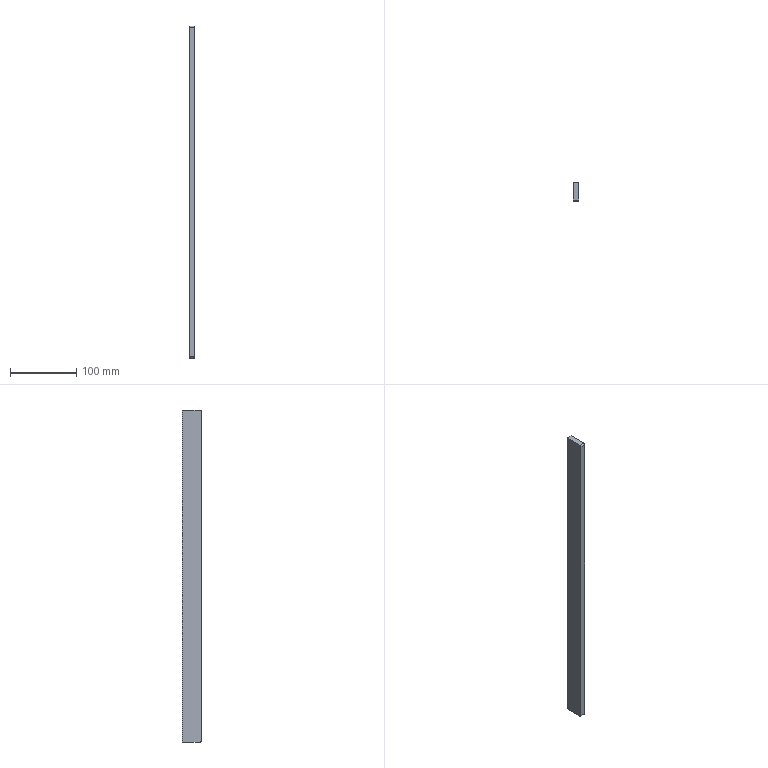Part | SolidWorks | features BaseBody 1 | 1 solid | 20 faces | box 8 x 29 x 500 mm | volume 115683 mm3 | cylinder 8 | cone 6 | plane 6 | commonest cylinder face diameters 3.3 x6 4 x2
STEP:
#1=CARTESIAN_POINT('',(-38.606,219.931,3066.293));
#2=VERTEX_POINT('',#1);
#3=CARTESIAN_POINT('',(-35.306,219.931,3066.293));
#4=VERTEX_POINT('',#3);
#5=CARTESIAN_POINT('',(-36.956,219.931,3066.293));
#6=DIRECTION('',(0.,1.,0.));
#7=DIRECTION('',(1.,0.,0.));
#8=AXIS2_PLACEMENT_3D('',#5,#6,#7);
#9=CIRCLE('',#8,1.65);
#10=EDGE_CURVE('',#2,#4,#9,.T.);
#11=ORIENTED_EDGE('',*,*,#10,.F.);
#12=CARTESIAN_POINT('',(-38.606,231.431,3066.293));
#13=VERTEX_POINT('',#12);
#14=CARTESIAN_POINT('',(-38.606,231.431,3066.293));
#15=DIRECTION('',(0.,1.,0.));
#16=VECTOR('',#15,1000.);
#17=LINE('',#14,#16);
#18=EDGE_CURVE('',#2,#13,#17,.T.);
#19=ORIENTED_EDGE('',*,*,#18,.T.);
#20=CARTESIAN_POINT('',(-35.306,231.431,3066.293));
#21=VERTEX_POINT('',#20);
#22=CARTESIAN_POINT('',(-36.956,231.431,3066.293));
#23=DIRECTION('',(0.,1.,0.));
#24=DIRECTION('',(1.,0.,0.));
#25=AXIS2_PLACEMENT_3D('',#22,#23,#24);
#26=CIRCLE('',#25,1.65);
#27=EDGE_CURVE('',#13,#21,#26,.T.);
#28=ORIENTED_EDGE('',*,*,#27,.T.);
#29=CARTESIAN_POINT('',(-35.306,231.431,3066.293));
#30=DIRECTION('',(0.,1.,0.));
#31=VECTOR('',#30,1000.);
#32=LINE('',#29,#31);
#33=EDGE_CURVE('',#4,#21,#32,.T.);
#34=ORIENTED_EDGE('',*,*,#33,.F.);
#35=EDGE_LOOP('',(#11,#19,#28,#34));
#36=FACE_OUTER_BOUND('',#35,.T.);
#37=CARTESIAN_POINT('',(-36.956,231.431,3066.293));
#38=DIRECTION('',(0.,1.,0.));
#39=DIRECTION('',(1.,0.,0.));
#40=AXIS2_PLACEMENT_3D('',#37,#38,#39);
#41=CYLINDRICAL_SURFACE('',#40,1.65);
#42=ADVANCED_FACE('',(#36),#41,.F.);
#43=CARTESIAN_POINT('',(-36.956,218.94,3066.293));
#44=VERTEX_POINT('',#43);
#45=CARTESIAN_POINT('',(-35.306,219.931,3066.293));
#46=DIRECTION('',(0.8572,0.515,0.));
#47=VECTOR('',#46,1000.);
#48=LINE('',#45,#47);
#49=EDGE_CURVE('',#44,#4,#48,.T.);
#50=ORIENTED_EDGE('',*,*,#49,.F.);
#51=CARTESIAN_POINT('',(-38.606,219.931,3066.293));
#52=DIRECTION('',(-0.8572,0.515,0.));
#53=VECTOR('',#52,1000.);
#54=LINE('',#51,#53);
#55=EDGE_CURVE('',#44,#2,#54,.T.);
#56=ORIENTED_EDGE('',*,*,#55,.T.);
#57=ORIENTED_EDGE('',*,*,#10,.T.);
#58=EDGE_LOOP('',(#50,#56,#57));
#59=FACE_OUTER_BOUND('',#58,.T.);
#60=CARTESIAN_POINT('',(-36.956,219.931,3066.293));
#61=DIRECTION('',(0.,1.,0.));
#62=DIRECTION('',(1.,0.,0.));
#63=AXIS2_PLACEMENT_3D('',#60,#61,#62);
#64=CONICAL_SURFACE('',#63,1.65,1.03);
#65=ADVANCED_FACE('',(#59),#64,.F.);
#66=CARTESIAN_POINT('',(-38.606,219.931,2596.293));
#67=VERTEX_POINT('',#66);
#68=CARTESIAN_POINT('',(-35.306,219.931,2596.293));
#69=VERTEX_POINT('',#68);
#70=CARTESIAN_POINT('',(-36.956,219.931,2596.293));
#71=DIRECTION('',(0.,1.,0.));
#72=DIRECTION('',(1.,0.,0.));
#73=AXIS2_PLACEMENT_3D('',#70,#71,#72);
#74=CIRCLE('',#73,1.65);
#75=EDGE_CURVE('',#67,#69,#74,.T.);
#76=ORIENTED_EDGE('',*,*,#75,.F.);
#77=CARTESIAN_POINT('',(-38.606,231.431,2596.293));
#78=VERTEX_POINT('',#77);
#79=CARTESIAN_POINT('',(-38.606,231.431,2596.293));
#80=DIRECTION('',(0.,1.,0.));
#81=VECTOR('',#80,1000.);
#82=LINE('',#79,#81);
#83=EDGE_CURVE('',#67,#78,#82,.T.);
#84=ORIENTED_EDGE('',*,*,#83,.T.);
#85=CARTESIAN_POINT('',(-35.306,231.431,2596.293));
#86=VERTEX_POINT('',#85);
#87=CARTESIAN_POINT('',(-36.956,231.431,2596.293));
#88=DIRECTION('',(0.,1.,0.));
#89=DIRECTION('',(1.,0.,0.));
#90=AXIS2_PLACEMENT_3D('',#87,#88,#89);
#91=CIRCLE('',#90,1.65);
#92=EDGE_CURVE('',#78,#86,#91,.T.);
#93=ORIENTED_EDGE('',*,*,#92,.T.);
#94=CARTESIAN_POINT('',(-35.306,231.431,2596.293));
#95=DIRECTION('',(0.,1.,0.));
#96=VECTOR('',#95,1000.);
#97=LINE('',#94,#96);
#98=EDGE_CURVE('',#69,#86,#97,.T.);
#99=ORIENTED_EDGE('',*,*,#98,.F.);
#100=EDGE_LOOP('',(#76,#84,#93,#99));
#101=FACE_OUTER_BOUND('',#100,.T.);
#102=CARTESIAN_POINT('',(-36.956,231.431,2596.293));
#103=DIRECTION('',(0.,1.,0.));
#104=DIRECTION('',(1.,0.,0.));
#105=AXIS2_PLACEMENT_3D('',#102,#103,#104);
#106=CYLINDRICAL_SURFACE('',#105,1.65);
#107=ADVANCED_FACE('',(#101),#106,.F.);
#108=CARTESIAN_POINT('',(-36.956,218.94,2596.293));
#109=VERTEX_POINT('',#108);
#110=CARTESIAN_POINT('',(-35.306,219.931,2596.293));
#111=DIRECTION('',(0.8572,0.515,0.));
#112=VECTOR('',#111,1000.);
#113=LINE('',#110,#112);
#114=EDGE_CURVE('',#109,#69,#113,.T.);
#115=ORIENTED_EDGE('',*,*,#114,.F.);
#116=CARTESIAN_POINT('',(-38.606,219.931,2596.293));
#117=DIRECTION('',(-0.8572,0.515,0.));
#118=VECTOR('',#117,1000.);
#119=LINE('',#116,#118);
#120=EDGE_CURVE('',#109,#67,#119,.T.);
#121=ORIENTED_EDGE('',*,*,#120,.T.);
#122=ORIENTED_EDGE('',*,*,#75,.T.);
#123=EDGE_LOOP('',(#115,#121,#122));
#124=FACE_OUTER_BOUND('',#123,.T.);
#125=CARTESIAN_POINT('',(-36.956,219.931,2596.293));
#126=DIRECTION('',(0.,1.,0.));
#127=DIRECTION('',(1.,0.,0.));
#128=AXIS2_PLACEMENT_3D('',#125,#126,#127);
#129=CONICAL_SURFACE('',#128,1.65,1.03);
#130=ADVANCED_FACE('',(#124),#129,.F.);
#131=CARTESIAN_POINT('',(-38.606,219.931,2888.793));
#132=VERTEX_POINT('',#131);
#133=CARTESIAN_POINT('',(-35.306,219.931,2888.793));
#134=VERTEX_POINT('',#133);
#135=CARTESIAN_POINT('',(-36.956,219.931,2888.793));
#136=DIRECTION('',(0.,1.,0.));
#137=DIRECTION('',(1.,0.,0.));
#138=AXIS2_PLACEMENT_3D('',#135,#136,#137);
#139=CIRCLE('',#138,1.65);
#140=EDGE_CURVE('',#132,#134,#139,.T.);
#141=ORIENTED_EDGE('',*,*,#140,.F.);
#142=CARTESIAN_POINT('',(-38.606,231.431,2888.793));
#143=VERTEX_POINT('',#142);
#144=CARTESIAN_POINT('',(-38.606,231.431,2888.793));
#145=DIRECTION('',(0.,1.,0.));
#146=VECTOR('',#145,1000.);
#147=LINE('',#144,#146);
#148=EDGE_CURVE('',#132,#143,#147,.T.);
#149=ORIENTED_EDGE('',*,*,#148,.T.);
#150=CARTESIAN_POINT('',(-35.306,231.431,2888.793));
#151=VERTEX_POINT('',#150);
#152=CARTESIAN_POINT('',(-36.956,231.431,2888.793));
#153=DIRECTION('',(0.,1.,0.));
#154=DIRECTION('',(1.,0.,0.));
#155=AXIS2_PLACEMENT_3D('',#152,#153,#154);
#156=CIRCLE('',#155,1.65);
#157=EDGE_CURVE('',#143,#151,#156,.T.);
#158=ORIENTED_EDGE('',*,*,#157,.T.);
#159=CARTESIAN_POINT('',(-35.306,231.431,2888.793));
#160=DIRECTION('',(0.,1.,0.));
#161=VECTOR('',#160,1000.);
#162=LINE('',#159,#161);
#163=EDGE_CURVE('',#134,#151,#162,.T.);
#164=ORIENTED_EDGE('',*,*,#163,.F.);
#165=EDGE_LOOP('',(#141,#149,#158,#164));
#166=FACE_OUTER_BOUND('',#165,.T.);
#167=CARTESIAN_POINT('',(-36.956,231.431,2888.793));
#168=DIRECTION('',(0.,1.,0.));
#169=DIRECTION('',(1.,0.,0.));
#170=AXIS2_PLACEMENT_3D('',#167,#168,#169);
#171=CYLINDRICAL_SURFACE('',#170,1.65);
#172=ADVANCED_FACE('',(#166),#171,.F.);
#173=CARTESIAN_POINT('',(-36.956,218.94,2888.793));
#174=VERTEX_POINT('',#173);
#175=CARTESIAN_POINT('',(-35.306,219.931,2888.793));
#176=DIRECTION('',(0.8572,0.515,0.));
#177=VECTOR('',#176,1000.);
#178=LINE('',#175,#177);
#179=EDGE_CURVE('',#174,#134,#178,.T.);
#180=ORIENTED_EDGE('',*,*,#179,.F.);
#181=CARTESIAN_POINT('',(-38.606,219.931,2888.793));
#182=DIRECTION('',(-0.8572,0.515,0.));
#183=VECTOR('',#182,1000.);
#184=LINE('',#181,#183);
#185=EDGE_CURVE('',#174,#132,#184,.T.);
#186=ORIENTED_EDGE('',*,*,#185,.T.);
#187=ORIENTED_EDGE('',*,*,#140,.T.);
#188=EDGE_LOOP('',(#180,#186,#187));
#189=FACE_OUTER_BOUND('',#188,.T.);
#190=CARTESIAN_POINT('',(-36.956,219.931,2888.793));
#191=DIRECTION('',(0.,1.,0.));
#192=DIRECTION('',(1.,0.,0.));
#193=AXIS2_PLACEMENT_3D('',#190,#191,#192);
#194=CONICAL_SURFACE('',#193,1.65,1.03);
#195=ADVANCED_FACE('',(#189),#194,.F.);
#196=CARTESIAN_POINT('',(-32.956,204.431,2581.293));
#197=VERTEX_POINT('',#196);
#198=CARTESIAN_POINT('',(-32.956,231.431,2581.293));
#199=VERTEX_POINT('',#198);
#200=CARTESIAN_POINT('',(-32.956,231.431,2581.293));
#201=DIRECTION('',(0.,1.,0.));
#202=VECTOR('',#201,1000.);
#203=LINE('',#200,#202);
#204=EDGE_CURVE('',#197,#199,#203,.T.);
#205=ORIENTED_EDGE('',*,*,#204,.F.);
#206=CARTESIAN_POINT('',(-40.956,204.431,2581.293));
#207=VERTEX_POINT('',#206);
#208=CARTESIAN_POINT('',(-32.956,204.431,2581.293));
#209=DIRECTION('',(-1.,0.,0.));
#210=VECTOR('',#209,1000.);
#211=LINE('',#208,#210);
#212=EDGE_CURVE('',#197,#207,#211,.T.);
#213=ORIENTED_EDGE('',*,*,#212,.T.);
#214=CARTESIAN_POINT('',(-40.956,231.431,2581.293));
#215=VERTEX_POINT('',#214);
#216=CARTESIAN_POINT('',(-40.956,231.431,2581.293));
#217=DIRECTION('',(0.,1.,0.));
#218=VECTOR('',#217,1000.);
#219=LINE('',#216,#218);
#220=EDGE_CURVE('',#207,#215,#219,.T.);
#221=ORIENTED_EDGE('',*,*,#220,.T.);
#222=CARTESIAN_POINT('',(-32.956,231.431,2581.293));
#223=DIRECTION('',(-1.,0.,0.));
#224=VECTOR('',#223,1000.);
#225=LINE('',#222,#224);
#226=EDGE_CURVE('',#199,#215,#225,.T.);
#227=ORIENTED_EDGE('',*,*,#226,.F.);
#228=EDGE_LOOP('',(#205,#213,#221,#227));
#229=FACE_OUTER_BOUND('',#228,.T.);
#230=CARTESIAN_POINT('',(-32.956,231.431,2581.293));
#231=DIRECTION('',(0.,0.,1.));
#232=DIRECTION('',(1.,0.,0.));
#233=AXIS2_PLACEMENT_3D('',#230,#231,#232);
#234=PLANE('',#233);
#235=ADVANCED_FACE('',(#229),#234,.F.);
#236=CARTESIAN_POINT('',(-40.956,231.431,3081.293));
#237=VERTEX_POINT('',#236);
#238=CARTESIAN_POINT('',(-40.956,231.431,3081.293));
#239=DIRECTION('',(0.,0.,1.));
#240=VECTOR('',#239,1000.);
#241=LINE('',#238,#240);
#242=EDGE_CURVE('',#215,#237,#241,.T.);
#243=ORIENTED_EDGE('',*,*,#242,.T.);
#244=CARTESIAN_POINT('',(-32.956,231.431,3081.293));
#245=VERTEX_POINT('',#244);
#246=CARTESIAN_POINT('',(-32.956,231.431,3081.293));
#247=DIRECTION('',(-1.,0.,0.));
#248=VECTOR('',#247,1000.);
#249=LINE('',#246,#248);
#250=EDGE_CURVE('',#245,#237,#249,.T.);
#251=ORIENTED_EDGE('',*,*,#250,.F.);
#252=CARTESIAN_POINT('',(-32.956,231.431,3081.293));
#253=DIRECTION('',(0.,0.,1.));
#254=VECTOR('',#253,1000.);
#255=LINE('',#252,#254);
#256=EDGE_CURVE('',#199,#245,#255,.T.);
#257=ORIENTED_EDGE('',*,*,#256,.F.);
#258=ORIENTED_EDGE('',*,*,#226,.T.);
#259=EDGE_LOOP('',(#243,#251,#257,#258));
#260=FACE_OUTER_BOUND('',#259,.T.);
#261=CARTESIAN_POINT('',(-36.956,231.431,3066.293));
#262=DIRECTION('',(0.,1.,0.));
#263=DIRECTION('',(1.,0.,0.));
#264=AXIS2_PLACEMENT_3D('',#261,#262,#263);
#265=CIRCLE('',#264,1.65);
#266=EDGE_CURVE('',#21,#13,#265,.T.);
#267=ORIENTED_EDGE('',*,*,#266,.F.);
#268=ORIENTED_EDGE('',*,*,#27,.F.);
#269=EDGE_LOOP('',(#267,#268));
#270=FACE_BOUND('',#269,.T.);
#271=CARTESIAN_POINT('',(-36.956,231.431,2596.293));
#272=DIRECTION('',(0.,1.,0.));
#273=DIRECTION('',(1.,0.,0.));
#274=AXIS2_PLACEMENT_3D('',#271,#272,#273);
#275=CIRCLE('',#274,1.65);
#276=EDGE_CURVE('',#86,#78,#275,.T.);
#277=ORIENTED_EDGE('',*,*,#276,.F.);
#278=ORIENTED_EDGE('',*,*,#92,.F.);
#279=EDGE_LOOP('',(#277,#278));
#280=FACE_BOUND('',#279,.T.);
#281=CARTESIAN_POINT('',(-36.956,231.431,2888.793));
#282=DIRECTION('',(0.,1.,0.));
#283=DIRECTION('',(1.,0.,0.));
#284=AXIS2_PLACEMENT_3D('',#281,#282,#283);
#285=CIRCLE('',#284,1.65);
#286=EDGE_CURVE('',#151,#143,#285,.T.);
#287=ORIENTED_EDGE('',*,*,#286,.F.);
#288=ORIENTED_EDGE('',*,*,#157,.F.);
#289=EDGE_LOOP('',(#287,#288));
#290=FACE_BOUND('',#289,.T.);
#291=CARTESIAN_POINT('',(-32.956,231.431,3081.293));
#292=DIRECTION('',(0.,-1.,0.));
#293=DIRECTION('',(-1.,0.,0.));
#294=AXIS2_PLACEMENT_3D('',#291,#292,#293);
#295=PLANE('',#294);
#296=ADVANCED_FACE('',(#260,#270,#280,#290),#295,.F.);
#297=CARTESIAN_POINT('',(-40.956,204.431,3081.293));
#298=VERTEX_POINT('',#297);
#299=CARTESIAN_POINT('',(-40.956,231.431,3081.293));
#300=DIRECTION('',(0.,-1.,0.));
#301=VECTOR('',#300,1000.);
#302=LINE('',#299,#301);
#303=EDGE_CURVE('',#237,#298,#302,.T.);
#304=ORIENTED_EDGE('',*,*,#303,.T.);
#305=CARTESIAN_POINT('',(-32.956,204.431,3081.293));
#306=VERTEX_POINT('',#305);
#307=CARTESIAN_POINT('',(-32.956,204.431,3081.293));
#308=DIRECTION('',(1.,0.,0.));
#309=VECTOR('',#308,1000.);
#310=LINE('',#307,#309);
#311=EDGE_CURVE('',#298,#306,#310,.T.);
#312=ORIENTED_EDGE('',*,*,#311,.T.);
#313=CARTESIAN_POINT('',(-32.956,231.431,3081.293));
#314=DIRECTION('',(0.,-1.,0.));
#315=VECTOR('',#314,1000.);
#316=LINE('',#313,#315);
#317=EDGE_CURVE('',#245,#306,#316,.T.);
#318=ORIENTED_EDGE('',*,*,#317,.F.);
#319=ORIENTED_EDGE('',*,*,#250,.T.);
#320=EDGE_LOOP('',(#304,#312,#318,#319));
#321=FACE_OUTER_BOUND('',#320,.T.);
#322=CARTESIAN_POINT('',(-32.956,231.431,3081.293));
#323=DIRECTION('',(0.,0.,-1.));
#324=DIRECTION('',(0.,1.,0.));
#325=AXIS2_PLACEMENT_3D('',#322,#323,#324);
#326=PLANE('',#325);
#327=ADVANCED_FACE('',(#321),#326,.F.);
#328=CARTESIAN_POINT('',(-40.956,202.431,3079.293));
#329=VERTEX_POINT('',#328);
#330=CARTESIAN_POINT('',(-40.956,202.431,2583.293));
#331=VERTEX_POINT('',#330);
#332=CARTESIAN_POINT('',(-40.956,202.431,3081.293));
#333=DIRECTION('',(0.,0.,-1.));
#334=VECTOR('',#333,1000.);
#335=LINE('',#332,#334);
#336=EDGE_CURVE('',#329,#331,#335,.T.);
#337=ORIENTED_EDGE('',*,*,#336,.T.);
#338=CARTESIAN_POINT('',(-32.956,202.431,2583.293));
#339=VERTEX_POINT('',#338);
#340=CARTESIAN_POINT('',(-32.956,202.431,2583.293));
#341=DIRECTION('',(1.,0.,0.));
#342=VECTOR('',#341,1000.);
#343=LINE('',#340,#342);
#344=EDGE_CURVE('',#331,#339,#343,.T.);
#345=ORIENTED_EDGE('',*,*,#344,.T.);
#346=CARTESIAN_POINT('',(-32.956,202.431,3079.293));
#347=VERTEX_POINT('',#346);
#348=CARTESIAN_POINT('',(-32.956,202.431,3081.293));
#349=DIRECTION('',(0.,0.,-1.));
#350=VECTOR('',#349,1000.);
#351=LINE('',#348,#350);
#352=EDGE_CURVE('',#347,#339,#351,.T.);
#353=ORIENTED_EDGE('',*,*,#352,.F.);
#354=CARTESIAN_POINT('',(-32.956,202.431,3079.293));
#355=DIRECTION('',(-1.,0.,0.));
#356=VECTOR('',#355,1000.);
#357=LINE('',#354,#356);
#358=EDGE_CURVE('',#347,#329,#357,.T.);
#359=ORIENTED_EDGE('',*,*,#358,.T.);
#360=EDGE_LOOP('',(#337,#345,#353,#359));
#361=FACE_OUTER_BOUND('',#360,.T.);
#362=CARTESIAN_POINT('',(-32.956,202.431,3081.293));
#363=DIRECTION('',(0.,1.,0.));
#364=DIRECTION('',(0.,0.,-1.));
#365=AXIS2_PLACEMENT_3D('',#362,#363,#364);
#366=PLANE('',#365);
#367=ADVANCED_FACE('',(#361),#366,.F.);
#368=ORIENTED_EDGE('',*,*,#352,.T.);
#369=CARTESIAN_POINT('',(-32.956,204.431,2583.293));
#370=DIRECTION('',(1.,0.,0.));
#371=DIRECTION('',(0.,0.,-1.));
#372=AXIS2_PLACEMENT_3D('',#369,#370,#371);
#373=CIRCLE('',#372,2.);
#374=EDGE_CURVE('',#339,#197,#373,.T.);
#375=ORIENTED_EDGE('',*,*,#374,.T.);
#376=ORIENTED_EDGE('',*,*,#204,.T.);
#377=ORIENTED_EDGE('',*,*,#256,.T.);
#378=ORIENTED_EDGE('',*,*,#317,.T.);
#379=CARTESIAN_POINT('',(-32.956,204.431,3079.293));
#380=DIRECTION('',(1.,0.,0.));
#381=DIRECTION('',(0.,0.,-1.));
#382=AXIS2_PLACEMENT_3D('',#379,#380,#381);
#383=CIRCLE('',#382,2.);
#384=EDGE_CURVE('',#306,#347,#383,.T.);
#385=ORIENTED_EDGE('',*,*,#384,.T.);
#386=EDGE_LOOP('',(#368,#375,#376,#377,#378,#385));
#387=FACE_OUTER_BOUND('',#386,.T.);
#388=CARTESIAN_POINT('',(-32.956,216.931,2831.293));
#389=DIRECTION('',(1.,0.,0.));
#390=DIRECTION('',(0.,0.,-1.));
#391=AXIS2_PLACEMENT_3D('',#388,#389,#390);
#392=PLANE('',#391);
#393=ADVANCED_FACE('',(#387),#392,.T.);
#394=ORIENTED_EDGE('',*,*,#220,.F.);
#395=CARTESIAN_POINT('',(-40.956,204.431,2583.293));
#396=DIRECTION('',(-1.,0.,0.));
#397=DIRECTION('',(0.,0.,-1.));
#398=AXIS2_PLACEMENT_3D('',#395,#396,#397);
#399=CIRCLE('',#398,2.);
#400=EDGE_CURVE('',#207,#331,#399,.T.);
#401=ORIENTED_EDGE('',*,*,#400,.T.);
#402=ORIENTED_EDGE('',*,*,#336,.F.);
#403=CARTESIAN_POINT('',(-40.956,204.431,3079.293));
#404=DIRECTION('',(-1.,0.,0.));
#405=DIRECTION('',(0.,0.,-1.));
#406=AXIS2_PLACEMENT_3D('',#403,#404,#405);
#407=CIRCLE('',#406,2.);
#408=EDGE_CURVE('',#329,#298,#407,.T.);
#409=ORIENTED_EDGE('',*,*,#408,.T.);
#410=ORIENTED_EDGE('',*,*,#303,.F.);
#411=ORIENTED_EDGE('',*,*,#242,.F.);
#412=EDGE_LOOP('',(#394,#401,#402,#409,#410,#411));
#413=FACE_OUTER_BOUND('',#412,.T.);
#414=CARTESIAN_POINT('',(-40.956,216.931,2831.293));
#415=DIRECTION('',(1.,0.,0.));
#416=DIRECTION('',(0.,0.,-1.));
#417=AXIS2_PLACEMENT_3D('',#414,#415,#416);
#418=PLANE('',#417);
#419=ADVANCED_FACE('',(#413),#418,.F.);
#420=ORIENTED_EDGE('',*,*,#185,.F.);
#421=ORIENTED_EDGE('',*,*,#179,.T.);
#422=CARTESIAN_POINT('',(-36.956,219.931,2888.793));
#423=DIRECTION('',(0.,1.,0.));
#424=DIRECTION('',(1.,0.,0.));
#425=AXIS2_PLACEMENT_3D('',#422,#423,#424);
#426=CIRCLE('',#425,1.65);
#427=EDGE_CURVE('',#134,#132,#426,.T.);
#428=ORIENTED_EDGE('',*,*,#427,.T.);
#429=EDGE_LOOP('',(#420,#421,#428));
#430=FACE_OUTER_BOUND('',#429,.T.);
#431=CARTESIAN_POINT('',(-36.956,219.931,2888.793));
#432=DIRECTION('',(0.,1.,0.));
#433=DIRECTION('',(1.,0.,0.));
#434=AXIS2_PLACEMENT_3D('',#431,#432,#433);
#435=CONICAL_SURFACE('',#434,1.65,1.03);
#436=ADVANCED_FACE('',(#430),#435,.F.);
#437=ORIENTED_EDGE('',*,*,#148,.F.);
#438=ORIENTED_EDGE('',*,*,#427,.F.);
#439=ORIENTED_EDGE('',*,*,#163,.T.);
#440=ORIENTED_EDGE('',*,*,#286,.T.);
#441=EDGE_LOOP('',(#437,#438,#439,#440));
#442=FACE_OUTER_BOUND('',#441,.T.);
#443=CARTESIAN_POINT('',(-36.956,231.431,2888.793));
#444=DIRECTION('',(0.,1.,0.));
#445=DIRECTION('',(1.,0.,0.));
#446=AXIS2_PLACEMENT_3D('',#443,#444,#445);
#447=CYLINDRICAL_SURFACE('',#446,1.65);
#448=ADVANCED_FACE('',(#442),#447,.F.);
#449=ORIENTED_EDGE('',*,*,#120,.F.);
#450=ORIENTED_EDGE('',*,*,#114,.T.);
#451=CARTESIAN_POINT('',(-36.956,219.931,2596.293));
#452=DIRECTION('',(0.,1.,0.));
#453=DIRECTION('',(1.,0.,0.));
#454=AXIS2_PLACEMENT_3D('',#451,#452,#453);
#455=CIRCLE('',#454,1.65);
#456=EDGE_CURVE('',#69,#67,#455,.T.);
#457=ORIENTED_EDGE('',*,*,#456,.T.);
#458=EDGE_LOOP('',(#449,#450,#457));
#459=FACE_OUTER_BOUND('',#458,.T.);
#460=CARTESIAN_POINT('',(-36.956,219.931,2596.293));
#461=DIRECTION('',(0.,1.,0.));
#462=DIRECTION('',(1.,0.,0.));
#463=AXIS2_PLACEMENT_3D('',#460,#461,#462);
#464=CONICAL_SURFACE('',#463,1.65,1.03);
#465=ADVANCED_FACE('',(#459),#464,.F.);
#466=ORIENTED_EDGE('',*,*,#83,.F.);
#467=ORIENTED_EDGE('',*,*,#456,.F.);
#468=ORIENTED_EDGE('',*,*,#98,.T.);
#469=ORIENTED_EDGE('',*,*,#276,.T.);
#470=EDGE_LOOP('',(#466,#467,#468,#469));
#471=FACE_OUTER_BOUND('',#470,.T.);
#472=CARTESIAN_POINT('',(-36.956,231.431,2596.293));
#473=DIRECTION('',(0.,1.,0.));
#474=DIRECTION('',(1.,0.,0.));
#475=AXIS2_PLACEMENT_3D('',#472,#473,#474);
#476=CYLINDRICAL_SURFACE('',#475,1.65);
#477=ADVANCED_FACE('',(#471),#476,.F.);
#478=ORIENTED_EDGE('',*,*,#55,.F.);
#479=ORIENTED_EDGE('',*,*,#49,.T.);
#480=CARTESIAN_POINT('',(-36.956,219.931,3066.293));
#481=DIRECTION('',(0.,1.,0.));
#482=DIRECTION('',(1.,0.,0.));
#483=AXIS2_PLACEMENT_3D('',#480,#481,#482);
#484=CIRCLE('',#483,1.65);
#485=EDGE_CURVE('',#4,#2,#484,.T.);
#486=ORIENTED_EDGE('',*,*,#485,.T.);
#487=EDGE_LOOP('',(#478,#479,#486));
#488=FACE_OUTER_BOUND('',#487,.T.);
#489=CARTESIAN_POINT('',(-36.956,219.931,3066.293));
#490=DIRECTION('',(0.,1.,0.));
#491=DIRECTION('',(1.,0.,0.));
#492=AXIS2_PLACEMENT_3D('',#489,#490,#491);
#493=CONICAL_SURFACE('',#492,1.65,1.03);
#494=ADVANCED_FACE('',(#488),#493,.F.);
#495=ORIENTED_EDGE('',*,*,#18,.F.);
#496=ORIENTED_EDGE('',*,*,#485,.F.);
#497=ORIENTED_EDGE('',*,*,#33,.T.);
#498=ORIENTED_EDGE('',*,*,#266,.T.);
#499=EDGE_LOOP('',(#495,#496,#497,#498));
#500=FACE_OUTER_BOUND('',#499,.T.);
#501=CARTESIAN_POINT('',(-36.956,231.431,3066.293));
#502=DIRECTION('',(0.,1.,0.));
#503=DIRECTION('',(1.,0.,0.));
#504=AXIS2_PLACEMENT_3D('',#501,#502,#503);
#505=CYLINDRICAL_SURFACE('',#504,1.65);
#506=ADVANCED_FACE('',(#500),#505,.F.);
#507=ORIENTED_EDGE('',*,*,#374,.F.);
#508=ORIENTED_EDGE('',*,*,#344,.F.);
#509=ORIENTED_EDGE('',*,*,#400,.F.);
#510=ORIENTED_EDGE('',*,*,#212,.F.);
#511=EDGE_LOOP('',(#507,#508,#509,#510));
#512=FACE_OUTER_BOUND('',#511,.T.);
#513=CARTESIAN_POINT('',(-32.956,204.431,2583.293));
#514=DIRECTION('',(-1.,0.,0.));
#515=DIRECTION('',(0.,0.,1.));
#516=AXIS2_PLACEMENT_3D('',#513,#514,#515);
#517=CYLINDRICAL_SURFACE('',#516,2.);
#518=ADVANCED_FACE('',(#512),#517,.T.);
#519=ORIENTED_EDGE('',*,*,#384,.F.);
#520=ORIENTED_EDGE('',*,*,#311,.F.);
#521=ORIENTED_EDGE('',*,*,#408,.F.);
#522=ORIENTED_EDGE('',*,*,#358,.F.);
#523=EDGE_LOOP('',(#519,#520,#521,#522));
#524=FACE_OUTER_BOUND('',#523,.T.);
#525=CARTESIAN_POINT('',(-32.956,204.431,3079.293));
#526=DIRECTION('',(-1.,0.,0.));
#527=DIRECTION('',(0.,0.,1.));
#528=AXIS2_PLACEMENT_3D('',#525,#526,#527);
#529=CYLINDRICAL_SURFACE('',#528,2.);
#530=ADVANCED_FACE('',(#524),#529,.T.);
#531=CLOSED_SHELL('',(#42,#65,#107,#130,#172,#195,#235,#296,#327,#367,#393,#419,#436,#448,#465,#477,#494,#506,#518,#530));
#532=MANIFOLD_SOLID_BREP('',#531);
#533=CARTESIAN_POINT('',(0.,0.,0.));
#534=DIRECTION('',(0.,0.,1.));
#535=DIRECTION('',(1.,0.,0.));
#536=AXIS2_PLACEMENT_3D('',#533,#534,#535);
#537=(LENGTH_UNIT()NAMED_UNIT(*)SI_UNIT(.MILLI.,.METRE.));
#538=UNCERTAINTY_MEASURE_WITH_UNIT(LENGTH_MEASURE(0.00001),#537,'','');
#539=(NAMED_UNIT(*)PLANE_ANGLE_UNIT()SI_UNIT($,.RADIAN.));
#540=(NAMED_UNIT(*)SI_UNIT($,.STERADIAN.)SOLID_ANGLE_UNIT());
#541=(GEOMETRIC_REPRESENTATION_CONTEXT(3)GLOBAL_UNCERTAINTY_ASSIGNED_CONTEXT((#538))GLOBAL_UNIT_ASSIGNED_CONTEXT((#537,#539,#540))REPRESENTATION_CONTEXT('',''));
#542=ADVANCED_BREP_SHAPE_REPRESENTATION('',(#532,#536),#541);